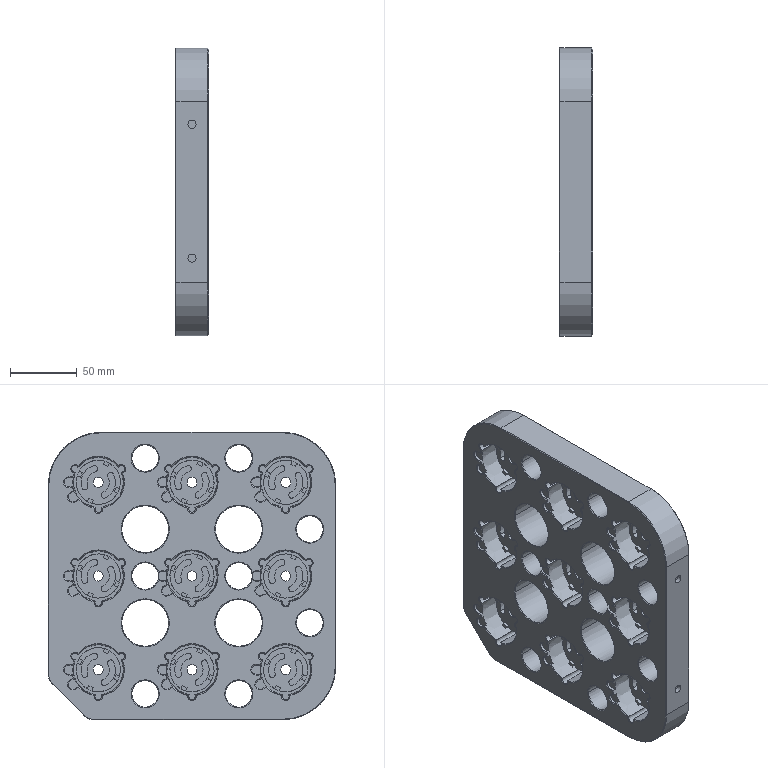Part | SolidWorks | features ICE 14, MoveCopyBody 7, LPattern 5, MoveFace 5, Chamfer 3, Cut 2, Stock 2, Extrusion 1, HoleWzd 1 | 1 solid | 781 faces | box 25 x 215 x 215 mm | volume 773722 mm3 | plane 325 | cone 237 | cylinder 219 | commonest cylinder face diameters 4 x90 7 x20 7.5 x18 16.55 x18 20 x18 25.656 x18